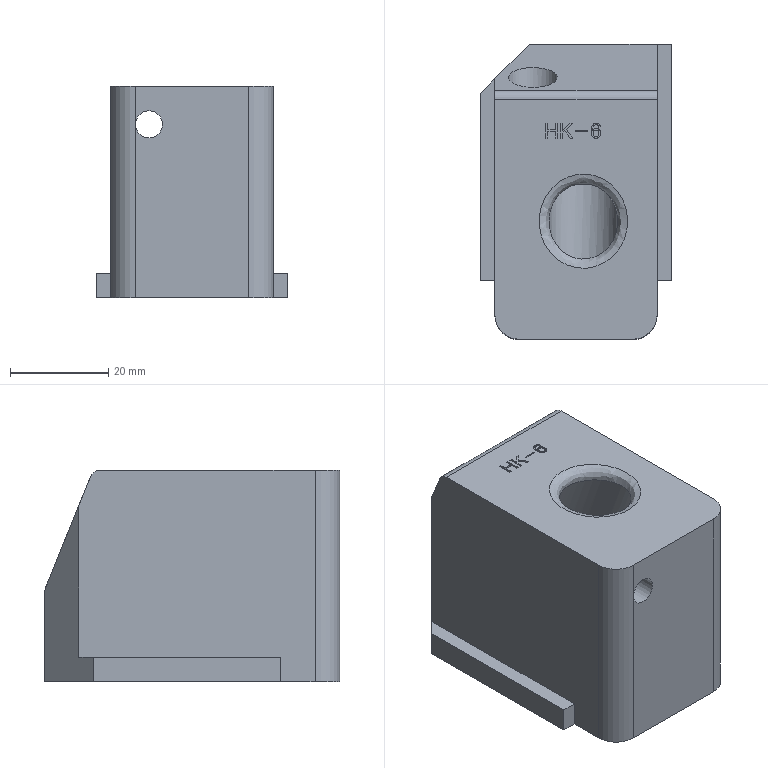Part | STEP file | solid 152 | 1 solid | 64 faces | box 39 x 60 x 43 mm | volume 71381 mm3 | plane 51 | cylinder 8 | other 4 | spline 1 | commonest cylinder face diameters 10 x3 4 x2 5.499 x1 6 x1 14 x1